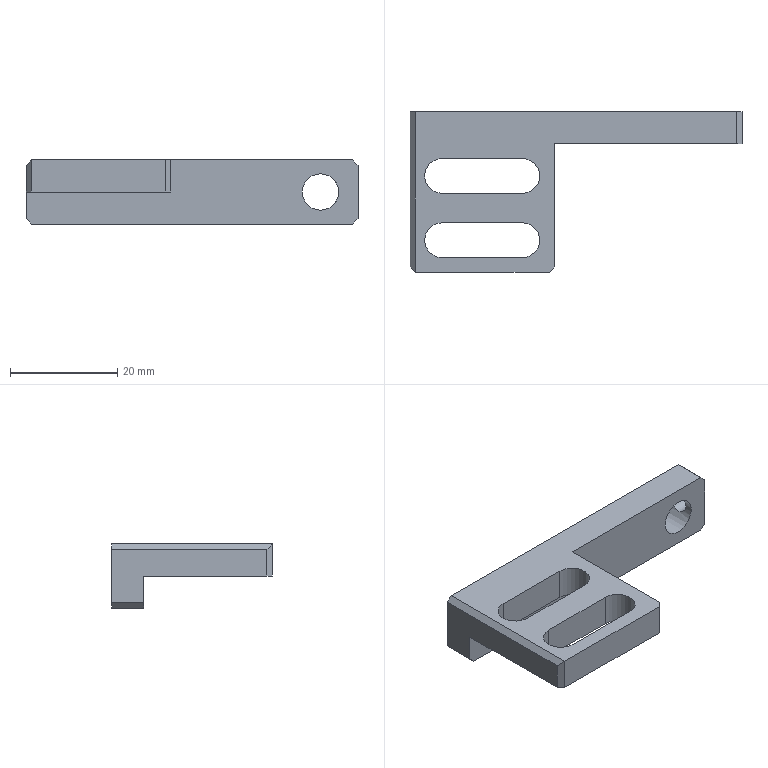NC program | NX | posted with a generic post | part box 62 x 30 x 12 mm
Lines 1128 to 2452 of 2452:
(ZLEVEL_PROFILE , TOOL : D4)
N2230 T11 M6
N2232 G54
N2234 G17 G0 G90 X11.003 Y1.75 S9500 M3
N2236 G43 Z30. H11
N2238 Z-5.
N2240 G94 G1 X25.158 Z-5.742 F1500.
N2242 X25.529 Y1.856 Z-5.762
N2244 X25.85 Y2.07 Z-5.782
N2246 X26.091 Y2.37 Z-5.802
N2248 X26.231 Y2.729 Z-5.823
N2250 X26.255 Y3.114 Z-5.843
N2252 X26.162 Y3.488 Z-5.863
N2254 X26.003 Y3.762 Z-5.88
N2256 X25.769 Y3.998 Z-5.897
N2258 X25.48 Y4.165 Z-5.915
N2260 X25.158 Y4.25 Z-5.932
N2262 X17.5 Z-6.333
N2264 X10.
N2266 G3 X8.75 Y3. R1.25
N2268 X10. Y1.75 R1.25
N2270 G1 X25.
N2272 G3 X26.25 Y3. R1.25
N2274 X25. Y4.25 R1.25
N2276 G1 X17.5
N2278 X10.198 Z-6.461
N2280 X10.058 Z-6.463
N2282 X9.918 Y4.239 Z-6.466
N2284 X9.716 Y4.209 Z-6.469
N2286 X9.643 Y4.193 Z-6.471
N2288 X9.51 Y4.143 Z-6.473
N2290 X9.388 Y4.081 Z-6.475
N2292 X9.242 Y3.984 Z-6.479
N2294 X9.16 Y3.92 Z-6.48
N2296 X9.063 Y3.818 Z-6.483
N2298 X8.979 Y3.708 Z-6.485
N2300 X8.89 Y3.557 Z-6.488
N2302 X8.844 Y3.464 Z-6.49
N2304 X8.804 Y3.335 Z-6.493
N2306 X8.773 Y3.194 Z-6.495
N2308 X8.752 Y3.075 Z-6.497
N2310 X8.753 Y2.915 Z-6.5
N2312 X8.803 Y2.64 Z-6.505
N2314 X8.913 Y2.382 Z-6.51
N2316 X8.983 Y2.287 Z-6.512
N2318 X9.084 Y2.161 Z-6.515
N2320 X9.205 Y2.045 Z-6.518
N2322 X9.292 Y1.975 Z-6.52
N2324 X9.416 Y1.903 Z-6.522
N2326 X9.54 Y1.846 Z-6.525
N2328 X9.696 Y1.795 Z-6.527
N2330 X9.808 Y1.77 Z-6.529
N2332 X9.947 Y1.758 Z-6.532
N2334 X10.087 Y1.75 Z-6.534
N2336 X17.67 Z-6.667
N2338 X25.
N2340 G3 X26.25 Y3. R1.25
N2342 X25. Y4.25 R1.25
N2344 G1 X17.5
N2346 X10.198 Z-6.794
N2348 X10.058 Z-6.797
N2350 X9.918 Y4.239 Z-6.799
N2352 X9.716 Y4.209 Z-6.803
N2354 X9.643 Y4.193 Z-6.804
N2356 X9.51 Y4.143 Z-6.806
N2358 X9.388 Y4.081 Z-6.809
N2360 X9.242 Y3.984 Z-6.812
N2362 X9.16 Y3.92 Z-6.814
N2364 X9.063 Y3.818 Z-6.816
N2366 X8.979 Y3.708 Z-6.819
N2368 X8.89 Y3.557 Z-6.822
N2370 X8.844 Y3.464 Z-6.824
N2372 X8.804 Y3.335 Z-6.826
N2374 X8.773 Y3.194 Z-6.828
N2376 X8.752 Y3.075 Z-6.831
N2378 X8.753 Y2.915 Z-6.833
N2380 X8.803 Y2.64 Z-6.838
N2382 X8.913 Y2.382 Z-6.843
N2384 X8.983 Y2.287 Z-6.845
N2386 X9.084 Y2.161 Z-6.848
N2388 X9.205 Y2.045 Z-6.851
N2390 X9.292 Y1.975 Z-6.853
N2392 X9.416 Y1.903 Z-6.855
N2394 X9.54 Y1.846 Z-6.858
N2396 X9.695 Y1.795 Z-6.861
N2398 X9.808 Y1.77 Z-6.863
N2400 X9.947 Y1.758 Z-6.865
N2402 X10.087 Y1.75 Z-6.868
N2404 X17.67 Z-7.
N2406 X25.
N2408 G3 X26.25 Y3. R1.25
N2410 X25. Y4.25 R1.25
N2412 G1 X17.5
N2414 X10.198 Z-7.127
N2416 X10.058 Z-7.13
N2418 X9.918 Y4.239 Z-7.132
N2420 X9.716 Y4.209 Z-7.136
N2422 X9.643 Y4.193 Z-7.137
N2424 X9.51 Y4.143 Z-7.14
N2426 X9.388 Y4.081 Z-7.142
N2428 X9.242 Y3.984 Z-7.145
N2430 X9.16 Y3.92 Z-7.147
N2432 X9.064 Y3.818 Z-7.15
N2434 X8.979 Y3.708 Z-7.152
N2436 X8.89 Y3.557 Z-7.155
N2438 X8.844 Y3.464 Z-7.157
N2440 X8.804 Y3.335 Z-7.159
N2442 X8.773 Y3.194 Z-7.162
N2444 X8.752 Y3.075 Z-7.164
N2446 X8.753 Y2.915 Z-7.167
N2448 X8.803 Y2.64 Z-7.172
N2450 X8.913 Y2.382 Z-7.176
N2452 X8.983 Y2.287 Z-7.179
N2454 X9.084 Y2.161 Z-7.181
N2456 X9.205 Y2.045 Z-7.184
N2458 X9.292 Y1.975 Z-7.186
N2460 X9.416 Y1.903 Z-7.189
N2462 X9.54 Y1.846 Z-7.191
N2464 X9.695 Y1.795 Z-7.194
N2466 X9.808 Y1.77 Z-7.196
N2468 X9.947 Y1.758 Z-7.199
N2470 X10.087 Y1.75 Z-7.201
N2472 X17.67 Z-7.333
N2474 X25.
N2476 G3 X26.25 Y3. R1.25
N2478 X25. Y4.25 R1.25
N2480 G1 X17.5
N2482 X10.198 Z-7.461
N2484 X10.058 Z-7.463
N2486 X9.918 Y4.239 Z-7.466
N2488 X9.716 Y4.209 Z-7.469
N2490 X9.643 Y4.193 Z-7.471
N2492 X9.51 Y4.143 Z-7.473
N2494 X9.388 Y4.081 Z-7.475
N2496 X9.242 Y3.984 Z-7.479
N2498 X9.16 Y3.92 Z-7.48
N2500 X9.064 Y3.818 Z-7.483
N2502 X8.979 Y3.708 Z-7.485
N2504 X8.89 Y3.557 Z-7.488
N2506 X8.844 Y3.464 Z-7.49
N2508 X8.804 Y3.335 Z-7.493
N2510 X8.773 Y3.194 Z-7.495
N2512 X8.752 Y3.075 Z-7.497
N2514 X8.753 Y2.915 Z-7.5
N2516 X8.803 Y2.64 Z-7.505
N2518 X8.913 Y2.382 Z-7.51
N2520 X8.983 Y2.287 Z-7.512
N2522 X9.084 Y2.161 Z-7.515
N2524 X9.205 Y2.045 Z-7.518
N2526 X9.292 Y1.975 Z-7.52
N2528 X9.416 Y1.903 Z-7.522
N2530 X9.54 Y1.846 Z-7.525
N2532 X9.695 Y1.795 Z-7.527
N2534 X9.808 Y1.77 Z-7.529
N2536 X9.947 Y1.758 Z-7.532
N2538 X10.087 Y1.75 Z-7.534
N2540 X17.67 Z-7.667
N2542 X25.
N2544 G3 X26.25 Y3. R1.25
N2546 X25. Y4.25 R1.25
N2548 G1 X17.5
N2550 X10.198 Z-7.794
N2552 X10.058 Z-7.797
N2554 X9.918 Y4.239 Z-7.799
N2556 X9.716 Y4.209 Z-7.803
N2558 X9.643 Y4.193 Z-7.804
N2560 X9.51 Y4.143 Z-7.806
N2562 X9.388 Y4.081 Z-7.809
N2564 X9.242 Y3.984 Z-7.812
N2566 X9.16 Y3.92 Z-7.814
N2568 X9.064 Y3.818 Z-7.816
N2570 X8.979 Y3.708 Z-7.819
N2572 X8.889 Y3.558 Z-7.822
N2574 X8.844 Y3.464 Z-7.824
N2576 X8.802 Y3.332 Z-7.826
N2578 X8.773 Y3.194 Z-7.828
N2580 X8.752 Y3.072 Z-7.831
N2582 X8.753 Y2.915 Z-7.833
N2584 X8.803 Y2.64 Z-7.838
N2586 X8.913 Y2.382 Z-7.843
N2588 X8.983 Y2.287 Z-7.845
N2590 X9.084 Y2.161 Z-7.848
N2592 X9.205 Y2.045 Z-7.851
N2594 X9.292 Y1.975 Z-7.853
N2596 X9.416 Y1.903 Z-7.855
N2598 X9.54 Y1.846 Z-7.858
N2600 X9.695 Y1.795 Z-7.861
N2602 X9.808 Y1.77 Z-7.863
N2604 X9.947 Y1.758 Z-7.865
N2606 X10.087 Y1.75 Z-7.868
N2608 X17.67 Z-8.
N2610 X25.
N2612 G3 X26.25 Y3. R1.25
N2614 X25. Y4.25 R1.25
N2616 G1 X17.5
N2618 X10.198 Z-8.127
N2620 X10.058 Z-8.13
N2622 X9.918 Y4.239 Z-8.132
N2624 X9.716 Y4.209 Z-8.136
N2626 X9.643 Y4.193 Z-8.137
N2628 X9.51 Y4.143 Z-8.14
N2630 X9.388 Y4.081 Z-8.142
N2632 X9.241 Y3.985 Z-8.145
N2634 X9.16 Y3.92 Z-8.147
N2636 X9.061 Y3.815 Z-8.15
N2638 X8.979 Y3.708 Z-8.152
N2640 X8.89 Y3.557 Z-8.155
N2642 X8.844 Y3.464 Z-8.157
N2644 X8.803 Y3.336 Z-8.159
N2646 X8.773 Y3.194 Z-8.162
N2648 X8.752 Y3.073 Z-8.164
N2650 X8.753 Y2.915 Z-8.167
N2652 X8.803 Y2.64 Z-8.172
N2654 X8.913 Y2.382 Z-8.176
N2656 X8.983 Y2.287 Z-8.179
N2658 X9.084 Y2.161 Z-8.181
N2660 X9.205 Y2.045 Z-8.184
N2662 X9.292 Y1.975 Z-8.186
N2664 X9.416 Y1.903 Z-8.189
N2666 X9.54 Y1.846 Z-8.191
N2668 X9.695 Y1.795 Z-8.194
N2670 X9.808 Y1.77 Z-8.196
N2672 X9.947 Y1.758 Z-8.199
N2674 X10.087 Y1.75 Z-8.201
N2676 X17.67 Z-8.333
N2678 X25.
N2680 G3 X26.25 Y3. R1.25
N2682 X25. Y4.25 R1.25
N2684 G1 X17.5
N2686 X10.198 Z-8.461
N2688 X10.058 Z-8.463
N2690 X9.918 Y4.239 Z-8.466
N2692 X9.716 Y4.209 Z-8.469
N2694 X9.643 Y4.193 Z-8.471
N2696 X9.51 Y4.143 Z-8.473
N2698 X9.388 Y4.081 Z-8.475
N2700 X9.241 Y3.985 Z-8.479
N2702 X9.16 Y3.92 Z-8.48
N2704 X9.061 Y3.815 Z-8.483
N2706 X8.979 Y3.708 Z-8.485
N2708 X8.89 Y3.557 Z-8.488
N2710 X8.844 Y3.464 Z-8.49
N2712 X8.803 Y3.336 Z-8.493
N2714 X8.773 Y3.194 Z-8.495
N2716 X8.752 Y3.073 Z-8.497
N2718 X8.753 Y2.915 Z-8.5
N2720 X8.803 Y2.64 Z-8.505
N2722 X8.913 Y2.382 Z-8.51
N2724 X8.983 Y2.287 Z-8.512
N2726 X9.084 Y2.161 Z-8.515
N2728 X9.205 Y2.045 Z-8.518
N2730 X9.292 Y1.975 Z-8.52
N2732 X9.416 Y1.903 Z-8.522
N2734 X9.54 Y1.846 Z-8.525
N2736 X9.695 Y1.795 Z-8.527
N2738 X9.808 Y1.77 Z-8.529
N2740 X9.947 Y1.758 Z-8.532
N2742 X10.087 Y1.75 Z-8.534
N2744 X17.67 Z-8.667
N2746 X25.
N2748 G3 X26.25 Y3. R1.25
N2750 X25. Y4.25 R1.25
N2752 G1 X17.5
N2754 X10.198 Z-8.794
N2756 X10.058 Z-8.797
N2758 X9.918 Y4.239 Z-8.799
N2760 X9.716 Y4.209 Z-8.803
N2762 X9.643 Y4.193 Z-8.804
N2764 X9.51 Y4.143 Z-8.806
N2766 X9.388 Y4.081 Z-8.809
N2768 X9.242 Y3.985 Z-8.812
N2770 X9.16 Y3.92 Z-8.814
N2772 X9.061 Y3.815 Z-8.816
N2774 X8.979 Y3.708 Z-8.819
N2776 X8.89 Y3.557 Z-8.822
N2778 X8.844 Y3.464 Z-8.824
N2780 X8.803 Y3.336 Z-8.826
N2782 X8.773 Y3.194 Z-8.828
N2784 X8.752 Y3.073 Z-8.831
N2786 X8.753 Y2.915 Z-8.833
N2788 X8.803 Y2.64 Z-8.838
N2790 X8.913 Y2.382 Z-8.843
N2792 X8.983 Y2.287 Z-8.845
N2794 X9.084 Y2.161 Z-8.848
N2796 X9.205 Y2.045 Z-8.851
N2798 X9.292 Y1.975 Z-8.853
N2800 X9.416 Y1.903 Z-8.855
N2802 X9.54 Y1.846 Z-8.858
N2804 X9.695 Y1.795 Z-8.861
N2806 X9.808 Y1.77 Z-8.863
N2808 X9.947 Y1.758 Z-8.865
N2810 X10.087 Y1.75 Z-8.868
N2812 X17.67 Z-9.
N2814 X25.
N2816 G3 X26.25 Y3. R1.25
N2818 X25. Y4.25 R1.25
N2820 G1 X17.5
N2822 X10.198 Z-9.127
N2824 X10.058 Z-9.13
N2826 X9.918 Y4.239 Z-9.132
N2828 X9.716 Y4.209 Z-9.136
N2830 X9.643 Y4.193 Z-9.137
N2832 X9.51 Y4.143 Z-9.14
N2834 X9.388 Y4.081 Z-9.142
N2836 X9.242 Y3.985 Z-9.145
N2838 X9.16 Y3.92 Z-9.147
N2840 X9.061 Y3.815 Z-9.15
N2842 X8.979 Y3.708 Z-9.152
N2844 X8.89 Y3.557 Z-9.155
N2846 X8.844 Y3.464 Z-9.157
N2848 X8.803 Y3.336 Z-9.159
N2850 X8.773 Y3.194 Z-9.162
N2852 X8.752 Y3.073 Z-9.164
N2854 X8.753 Y2.915 Z-9.167
N2856 X8.803 Y2.64 Z-9.172
N2858 X8.913 Y2.382 Z-9.176
N2860 X8.983 Y2.287 Z-9.179
N2862 X9.084 Y2.161 Z-9.181
N2864 X9.205 Y2.045 Z-9.184
N2866 X9.292 Y1.975 Z-9.186
N2868 X9.416 Y1.903 Z-9.189
N2870 X9.54 Y1.846 Z-9.191
N2872 X9.695 Y1.795 Z-9.194
N2874 X9.808 Y1.77 Z-9.196
N2876 X9.947 Y1.758 Z-9.199
N2878 X10.087 Y1.75 Z-9.201
N2880 X17.67 Z-9.333
N2882 X25.
N2884 G3 X26.25 Y3. R1.25
N2886 X25. Y4.25 R1.25
N2888 G1 X17.5
N2890 X10.198 Z-9.461
N2892 X10.058 Z-9.463
N2894 X9.918 Y4.239 Z-9.466
N2896 X9.716 Y4.209 Z-9.469
N2898 X9.643 Y4.193 Z-9.471
N2900 X9.51 Y4.143 Z-9.473
N2902 X9.388 Y4.081 Z-9.475
N2904 X9.242 Y3.985 Z-9.479
N2906 X9.16 Y3.92 Z-9.48
N2908 X9.061 Y3.815 Z-9.483
N2910 X8.979 Y3.708 Z-9.485
N2912 X8.89 Y3.557 Z-9.488
N2914 X8.844 Y3.464 Z-9.49
N2916 X8.803 Y3.336 Z-9.493
N2918 X8.773 Y3.194 Z-9.495
N2920 X8.752 Y3.073 Z-9.497
N2922 X8.753 Y2.915 Z-9.5
N2924 X8.803 Y2.64 Z-9.505
N2926 X8.913 Y2.382 Z-9.51
N2928 X8.983 Y2.287 Z-9.512
N2930 X9.084 Y2.161 Z-9.515
N2932 X9.205 Y2.045 Z-9.518
N2934 X9.292 Y1.975 Z-9.52
N2936 X9.416 Y1.903 Z-9.522
N2938 X9.54 Y1.846 Z-9.525
N2940 X9.695 Y1.795 Z-9.527
N2942 X9.808 Y1.77 Z-9.529
N2944 X9.947 Y1.758 Z-9.532
N2946 X10.087 Y1.75 Z-9.534
N2948 X17.67 Z-9.667
N2950 X25.
N2952 G3 X26.25 Y3. R1.25
N2954 X25. Y4.25 R1.25
N2956 G1 X17.5
N2958 X10.198 Z-9.794
N2960 X10.058 Z-9.797
N2962 X9.918 Y4.239 Z-9.799
N2964 X9.716 Y4.209 Z-9.803
N2966 X9.643 Y4.193 Z-9.804
N2968 X9.51 Y4.143 Z-9.806
N2970 X9.388 Y4.081 Z-9.809
N2972 X9.242 Y3.985 Z-9.812
N2974 X9.16 Y3.92 Z-9.814
N2976 X9.061 Y3.815 Z-9.816
N2978 X8.979 Y3.708 Z-9.819
N2980 X8.889 Y3.557 Z-9.822
N2982 X8.844 Y3.464 Z-9.824
N2984 X8.802 Y3.332 Z-9.826
N2986 X8.773 Y3.194 Z-9.828
N2988 X8.752 Y3.072 Z-9.831
N2990 X8.753 Y2.915 Z-9.833
N2992 X8.803 Y2.64 Z-9.838
N2994 X8.913 Y2.382 Z-9.843
N2996 X8.983 Y2.287 Z-9.845
N2998 X9.084 Y2.161 Z-9.848
N3000 X9.205 Y2.045 Z-9.851
N3002 X9.292 Y1.975 Z-9.853
N3004 X9.415 Y1.903 Z-9.855
N3006 X9.54 Y1.846 Z-9.858
N3008 X9.695 Y1.795 Z-9.861
N3010 X9.808 Y1.77 Z-9.863
N3012 X9.947 Y1.758 Z-9.865
N3014 X10.087 Y1.75 Z-9.868
N3016 X17.67 Z-10.
N3018 X25.
N3020 G3 X26.25 Y3. R1.25
N3022 X25. Y4.25 R1.25
N3024 G1 X17.5
N3026 X10.198 Z-10.127
N3028 X10.058 Z-10.13
N3030 X9.918 Y4.239 Z-10.132
N3032 X9.716 Y4.209 Z-10.136
N3034 X9.643 Y4.193 Z-10.137
N3036 X9.51 Y4.143 Z-10.14
N3038 X9.388 Y4.081 Z-10.142
N3040 X9.242 Y3.985 Z-10.145
N3042 X9.16 Y3.92 Z-10.147
N3044 X9.061 Y3.815 Z-10.15
N3046 X8.979 Y3.708 Z-10.152
N3048 X8.889 Y3.557 Z-10.155
N3050 X8.844 Y3.464 Z-10.157
N3052 X8.802 Y3.332 Z-10.159
N3054 X8.773 Y3.194 Z-10.162
N3056 X8.752 Y3.072 Z-10.164
N3058 X8.753 Y2.915 Z-10.167
N3060 X8.803 Y2.64 Z-10.172
N3062 X8.913 Y2.382 Z-10.176
N3064 X8.983 Y2.287 Z-10.179
N3066 X9.084 Y2.161 Z-10.181
N3068 X9.205 Y2.045 Z-10.184
N3070 X9.292 Y1.975 Z-10.186
N3072 X9.415 Y1.903 Z-10.189
N3074 X9.54 Y1.846 Z-10.191
N3076 X9.695 Y1.795 Z-10.194
N3078 X9.808 Y1.77 Z-10.196
N3080 X9.947 Y1.758 Z-10.199
N3082 X10.087 Y1.75 Z-10.201
N3084 X17.67 Z-10.333
N3086 X25.
N3088 G3 X26.25 Y3. R1.25
N3090 X25. Y4.25 R1.25
N3092 G1 X17.5
N3094 X10.198 Z-10.461
N3096 X10.058 Z-10.463
N3098 X9.918 Y4.239 Z-10.466
N3100 X9.716 Y4.209 Z-10.469
N3102 X9.643 Y4.193 Z-10.471
N3104 X9.51 Y4.143 Z-10.473
N3106 X9.388 Y4.081 Z-10.475
N3108 X9.242 Y3.985 Z-10.479
N3110 X9.16 Y3.92 Z-10.48
N3112 X9.061 Y3.815 Z-10.483
N3114 X8.979 Y3.708 Z-10.485
N3116 X8.889 Y3.557 Z-10.488
N3118 X8.844 Y3.464 Z-10.49
N3120 X8.802 Y3.332 Z-10.493
N3122 X8.773 Y3.194 Z-10.495
N3124 X8.752 Y3.072 Z-10.497
N3126 X8.753 Y2.915 Z-10.5
N3128 X8.803 Y2.64 Z-10.505
N3130 X8.913 Y2.382 Z-10.51
N3132 X8.983 Y2.287 Z-10.512
N3134 X9.084 Y2.161 Z-10.515
N3136 X9.205 Y2.045 Z-10.518
N3138 X9.292 Y1.975 Z-10.52
N3140 X9.415 Y1.903 Z-10.522
N3142 X9.54 Y1.846 Z-10.525
N3144 X9.695 Y1.795 Z-10.527
N3146 X9.808 Y1.77 Z-10.529
N3148 X9.947 Y1.758 Z-10.532
N3150 X10.087 Y1.75 Z-10.534
N3152 X17.67 Z-10.667
N3154 X25.
N3156 G3 X26.25 Y3. R1.25
N3158 X25. Y4.25 R1.25
N3160 G1 X17.5
N3162 X10.198 Z-10.794
N3164 X10.058 Z-10.797
N3166 X9.918 Y4.239 Z-10.799
N3168 X9.716 Y4.209 Z-10.803
N3170 X9.643 Y4.193 Z-10.804
N3172 X9.51 Y4.143 Z-10.806
N3174 X9.388 Y4.081 Z-10.809
N3176 X9.242 Y3.985 Z-10.812
N3178 X9.16 Y3.92 Z-10.814
N3180 X9.061 Y3.815 Z-10.816
N3182 X8.979 Y3.708 Z-10.819
N3184 X8.889 Y3.557 Z-10.822
N3186 X8.844 Y3.464 Z-10.824
N3188 X8.802 Y3.332 Z-10.826
N3190 X8.773 Y3.194 Z-10.828
N3192 X8.752 Y3.072 Z-10.831
N3194 X8.753 Y2.915 Z-10.833
N3196 X8.803 Y2.64 Z-10.838
N3198 X8.913 Y2.382 Z-10.843
N3200 X8.983 Y2.287 Z-10.845
N3202 X9.084 Y2.161 Z-10.848
N3204 X9.205 Y2.045 Z-10.851
N3206 X9.292 Y1.975 Z-10.853
N3208 X9.415 Y1.903 Z-10.855
N3210 X9.54 Y1.846 Z-10.858
N3212 X9.695 Y1.795 Z-10.861
N3214 X9.808 Y1.77 Z-10.863
N3216 X9.947 Y1.758 Z-10.865
N3218 X10.087 Y1.75 Z-10.868
N3220 X17.67 Z-11.
N3222 X25.
N3224 G3 X26.25 Y3. R1.25
N3226 X25. Y4.25 R1.25
N3228 G1 X17.5
N3230 X10.198 Z-11.127
N3232 X10.058 Z-11.13
N3234 X9.918 Y4.239 Z-11.132
N3236 X9.716 Y4.209 Z-11.136
N3238 X9.643 Y4.193 Z-11.137
N3240 X9.51 Y4.143 Z-11.14
N3242 X9.388 Y4.081 Z-11.142
N3244 X9.242 Y3.985 Z-11.145
N3246 X9.16 Y3.92 Z-11.147
N3248 X9.061 Y3.815 Z-11.15
N3250 X8.979 Y3.708 Z-11.152
N3252 X8.889 Y3.557 Z-11.155
N3254 X8.844 Y3.464 Z-11.157
N3256 X8.802 Y3.332 Z-11.159
N3258 X8.773 Y3.194 Z-11.162
N3260 X8.752 Y3.072 Z-11.164
N3262 X8.753 Y2.915 Z-11.167
N3264 X8.803 Y2.64 Z-11.172
N3266 X8.913 Y2.382 Z-11.176
N3268 X8.983 Y2.287 Z-11.179
N3270 X9.084 Y2.161 Z-11.181
N3272 X9.205 Y2.045 Z-11.184
N3274 X9.292 Y1.975 Z-11.186
N3276 X9.415 Y1.903 Z-11.189
N3278 X9.54 Y1.846 Z-11.191
N3280 X9.695 Y1.795 Z-11.194
N3282 X9.808 Y1.77 Z-11.196
N3284 X9.947 Y1.758 Z-11.199
N3286 X10.087 Y1.75 Z-11.201
N3288 X17.67 Z-11.333
N3290 X25.
N3292 G3 X26.25 Y3. R1.25
N3294 X25. Y4.25 R1.25
N3296 G1 X17.5
N3298 X10.198 Z-11.461
N3300 X10.058 Z-11.463
N3302 X9.918 Y4.239 Z-11.466
N3304 X9.716 Y4.209 Z-11.469
N3306 X9.643 Y4.193 Z-11.471
N3308 X9.51 Y4.143 Z-11.473
N3310 X9.388 Y4.081 Z-11.475
N3312 X9.242 Y3.985 Z-11.479
N3314 X9.16 Y3.92 Z-11.48
N3316 X9.061 Y3.815 Z-11.483
N3318 X8.979 Y3.708 Z-11.485
N3320 X8.889 Y3.557 Z-11.488
N3322 X8.844 Y3.464 Z-11.49
N3324 X8.802 Y3.332 Z-11.493
N3326 X8.773 Y3.194 Z-11.495
N3328 X8.752 Y3.072 Z-11.497
N3330 X8.753 Y2.915 Z-11.5
N3332 X8.803 Y2.64 Z-11.505
N3334 X8.913 Y2.382 Z-11.51
N3336 X8.983 Y2.287 Z-11.512
N3338 X9.084 Y2.161 Z-11.515
N3340 X9.205 Y2.045 Z-11.518
N3342 X9.292 Y1.975 Z-11.52
N3344 X9.415 Y1.903 Z-11.522
N3346 X9.54 Y1.846 Z-11.525
N3348 X9.695 Y1.795 Z-11.527
N3350 X9.808 Y1.77 Z-11.529
N3352 X9.947 Y1.758 Z-11.532
N3354 X10.087 Y1.75 Z-11.534
N3356 X17.67 Z-11.667
N3358 X25.
N3360 G3 X26.25 Y3. R1.25
N3362 X25. Y4.25 R1.25
N3364 G1 X17.5
N3366 X10.198 Z-11.794
N3368 X10.058 Z-11.797
N3370 X9.918 Y4.239 Z-11.799
N3372 X9.716 Y4.209 Z-11.803
N3374 X9.643 Y4.193 Z-11.804
N3376 X9.51 Y4.143 Z-11.806
N3378 X9.388 Y4.081 Z-11.809
N3380 X9.242 Y3.985 Z-11.812
N3382 X9.16 Y3.92 Z-11.814
N3384 X9.061 Y3.815 Z-11.816
N3386 X8.979 Y3.708 Z-11.819
N3388 X8.889 Y3.557 Z-11.822
N3390 X8.844 Y3.464 Z-11.824
N3392 X8.802 Y3.332 Z-11.826
N3394 X8.773 Y3.194 Z-11.828
N3396 X8.752 Y3.072 Z-11.831
N3398 X8.753 Y2.915 Z-11.833
N3400 X8.803 Y2.64 Z-11.838
N3402 X8.913 Y2.382 Z-11.843
N3404 X8.983 Y2.287 Z-11.845
N3406 X9.084 Y2.161 Z-11.848
N3408 X9.205 Y2.045 Z-11.851
N3410 X9.292 Y1.975 Z-11.853
N3412 X9.415 Y1.903 Z-11.855
N3414 X9.54 Y1.846 Z-11.858
N3416 X9.695 Y1.795 Z-11.861
N3418 X9.808 Y1.77 Z-11.863
N3420 X9.947 Y1.758 Z-11.865
N3422 X10.087 Y1.75 Z-11.868
N3424 X17.67 Z-12.
N3426 X25.
N3428 G3 X26.25 Y3. R1.25
N3430 X25. Y4.25 R1.25
N3432 G1 X10.
N3434 G3 X8.75 Y3. R1.25
N3436 X10. Y1.75 R1.25
N3438 G1 X17.67
N3440 Z-11.
N3442 G0 Z30.
N3444 X24. Y-7.75
N3446 Z-5.
N3448 G1 X9.842 Z-5.742
N3450 X9.479 Y-7.853 Z-5.762
N3452 X9.162 Y-8.059 Z-5.782
N3454 X8.921 Y-8.349 Z-5.801
N3456 X8.793 Y-8.639 Z-5.818
N3458 X8.742 Y-9.071 Z-5.841
N3460 X8.841 Y-9.495 Z-5.864
N3462 X9.079 Y-9.859 Z-5.886
N3464 X9.426 Y-10.122 Z-5.909
N3466 X9.842 Y-10.25 Z-5.932
N3468 X17.5 Z-6.333
N3470 X25.
N3472 G3 X26.25 Y-9. R1.25
N3474 X25. Y-7.75 R1.25
N3476 G1 X10.
N3478 G3 X8.75 Y-9. R1.25
N3480 X10. Y-10.25 R1.25
N3482 G1 X17.5
N3484 X24.802 Z-6.461
N3486 X24.942 Z-6.463
N3488 X25.082 Y-10.239 Z-6.466
N3490 X25.284 Y-10.209 Z-6.469
N3492 X25.357 Y-10.193 Z-6.471
N3494 X25.49 Y-10.143 Z-6.473
N3496 X25.612 Y-10.081 Z-6.475
N3498 X25.758 Y-9.984 Z-6.479
N3500 X25.84 Y-9.92 Z-6.48
N3502 X25.937 Y-9.818 Z-6.483
N3504 X26.021 Y-9.708 Z-6.485
N3506 X26.11 Y-9.557 Z-6.488
N3508 X26.156 Y-9.464 Z-6.49
N3510 X26.199 Y-9.33 Z-6.493
N3512 X26.227 Y-9.194 Z-6.495
N3514 X26.242 Y-9.02 Z-6.498
N3516 Y-8.916 Z-6.5
N3518 X26.223 Y-8.776 Z-6.502
N3520 X26.189 Y-8.642 Z-6.505
N3522 X26.127 Y-8.478 Z-6.508
N3524 X26.082 Y-8.384 Z-6.51
N3526 X26.004 Y-8.267 Z-6.512
N3528 X25.916 Y-8.161 Z-6.515
N3530 X25.789 Y-8.041 Z-6.518
N3532 X25.708 Y-7.975 Z-6.52
N3534 X25.586 Y-7.904 Z-6.522
N3536 X25.46 Y-7.846 Z-6.525
N3538 X25.305 Y-7.795 Z-6.527
N3540 X25.192 Y-7.77 Z-6.529
N3542 X25.053 Y-7.758 Z-6.532
N3544 X24.913 Y-7.75 Z-6.534
N3546 X17.33 Z-6.667
N3548 X10.
N3550 G3 X8.75 Y-9. R1.25
N3552 X10. Y-10.25 R1.25
N3554 G1 X17.5
N3556 X24.802 Z-6.794
N3558 X24.942 Z-6.797
N3560 X25.082 Y-10.239 Z-6.799
N3562 X25.284 Y-10.209 Z-6.803
N3564 X25.357 Y-10.193 Z-6.804
N3566 X25.49 Y-10.143 Z-6.806
N3568 X25.612 Y-10.081 Z-6.809
N3570 X25.758 Y-9.984 Z-6.812
N3572 X25.84 Y-9.92 Z-6.814
N3574 X25.937 Y-9.818 Z-6.816
N3576 X26.021 Y-9.708 Z-6.819
N3578 X26.11 Y-9.557 Z-6.822
N3580 X26.156 Y-9.464 Z-6.824
N3582 X26.199 Y-9.33 Z-6.826
N3584 X26.227 Y-9.194 Z-6.828
N3586 X26.242 Y-9.02 Z-6.831
N3588 Y-8.916 Z-6.833
N3590 X26.223 Y-8.776 Z-6.836
N3592 X26.189 Y-8.642 Z-6.838
N3594 X26.127 Y-8.478 Z-6.841
N3596 X26.082 Y-8.384 Z-6.843
N3598 X26.004 Y-8.267 Z-6.846
N3600 X25.916 Y-8.161 Z-6.848
N3602 X25.789 Y-8.041 Z-6.851
N3604 X25.708 Y-7.975 Z-6.853
N3606 X25.586 Y-7.904 Z-6.855
N3608 X25.46 Y-7.846 Z-6.858
N3610 X25.305 Y-7.795 Z-6.861
N3612 X25.192 Y-7.77 Z-6.863
N3614 X25.053 Y-7.758 Z-6.865
N3616 X24.913 Y-7.75 Z-6.868
N3618 X17.33 Z-7.
N3620 X10.
N3622 G3 X8.75 Y-9. R1.25
N3624 X10. Y-10.25 R1.25
N3626 G1 X17.5
N3628 X24.802 Z-7.127
N3630 X24.942 Z-7.13
N3632 X25.082 Y-10.239 Z-7.132
N3634 X25.284 Y-10.209 Z-7.136
N3636 X25.357 Y-10.193 Z-7.137
N3638 X25.49 Y-10.143 Z-7.14
N3640 X25.612 Y-10.081 Z-7.142
N3642 X25.758 Y-9.984 Z-7.145
N3644 X25.84 Y-9.92 Z-7.147
N3646 X25.936 Y-9.818 Z-7.15
N3648 X26.021 Y-9.708 Z-7.152
N3650 X26.11 Y-9.557 Z-7.155
N3652 X26.156 Y-9.464 Z-7.157
N3654 X26.199 Y-9.33 Z-7.159
N3656 X26.227 Y-9.194 Z-7.162
N3658 X26.242 Y-9.02 Z-7.165
N3660 Y-8.916 Z-7.167
N3662 X26.223 Y-8.776 Z-7.169
N3664 X26.189 Y-8.642 Z-7.172
N3666 X26.127 Y-8.478 Z-7.175
N3668 X26.082 Y-8.384 Z-7.176
N3670 X26.004 Y-8.267 Z-7.179
N3672 X25.916 Y-8.161 Z-7.181
N3674 X25.789 Y-8.041 Z-7.184
N3676 X25.708 Y-7.975 Z-7.186
N3678 X25.586 Y-7.904 Z-7.189
N3680 X25.46 Y-7.846 Z-7.191
N3682 X25.305 Y-7.795 Z-7.194
N3684 X25.192 Y-7.77 Z-7.196
N3686 X25.053 Y-7.758 Z-7.199
N3688 X24.913 Y-7.75 Z-7.201
N3690 X17.33 Z-7.333
N3692 X10.
N3694 G3 X8.75 Y-9. R1.25
N3696 X10. Y-10.25 R1.25
N3698 G1 X17.5
N3700 X24.802 Z-7.461
N3702 X24.942 Z-7.463
N3704 X25.082 Y-10.239 Z-7.466
N3706 X25.284 Y-10.209 Z-7.469
N3708 X25.357 Y-10.193 Z-7.471
N3710 X25.49 Y-10.143 Z-7.473
N3712 X25.612 Y-10.081 Z-7.475
N3714 X25.758 Y-9.984 Z-7.479
N3716 X25.84 Y-9.92 Z-7.48
N3718 X25.936 Y-9.818 Z-7.483
N3720 X26.021 Y-9.708 Z-7.485
N3722 X26.11 Y-9.557 Z-7.488
N3724 X26.156 Y-9.464 Z-7.49
N3726 X26.199 Y-9.33 Z-7.493
N3728 X26.227 Y-9.194 Z-7.495
N3730 X26.242 Y-9.02 Z-7.498
N3732 Y-8.916 Z-7.5
N3734 X26.223 Y-8.776 Z-7.502
N3736 X26.189 Y-8.642 Z-7.505
N3738 X26.127 Y-8.479 Z-7.508
N3740 X26.082 Y-8.384 Z-7.51
N3742 X26.004 Y-8.267 Z-7.512
N3744 X25.916 Y-8.161 Z-7.515
N3746 X25.789 Y-8.041 Z-7.518
N3748 X25.708 Y-7.975 Z-7.52
N3750 X25.586 Y-7.904 Z-7.522
N3752 X25.46 Y-7.846 Z-7.525
N3754 X25.305 Y-7.795 Z-7.527
N3756 X25.192 Y-7.77 Z-7.529
N3758 X25.053 Y-7.758 Z-7.532
N3760 X24.913 Y-7.75 Z-7.534
N3762 X17.33 Z-7.667
N3764 X10.
N3766 G3 X8.75 Y-9. R1.25
N3768 X10. Y-10.25 R1.25
N3770 G1 X17.5
N3772 X24.802 Z-7.794
N3774 X24.942 Z-7.797
N3776 X25.082 Y-10.239 Z-7.799
N3778 X25.284 Y-10.209 Z-7.803
N3780 X25.357 Y-10.193 Z-7.804
N3782 X25.49 Y-10.143 Z-7.806
N3784 X25.612 Y-10.081 Z-7.809
N3786 X25.758 Y-9.984 Z-7.812
N3788 X25.84 Y-9.92 Z-7.814
N3790 X25.936 Y-9.818 Z-7.816
N3792 X26.021 Y-9.708 Z-7.819
N3794 X26.111 Y-9.558 Z-7.822
N3796 X26.156 Y-9.464 Z-7.824
N3798 X26.2 Y-9.326 Z-7.826
N3800 X26.227 Y-9.194 Z-7.828
N3802 X26.242 Y-9.019 Z-7.832
N3804 Y-8.916 Z-7.833
N3806 X26.223 Y-8.776 Z-7.836
N3808 X26.189 Y-8.642 Z-7.838
N3810 X26.127 Y-8.479 Z-7.841
N3812 X26.082 Y-8.384 Z-7.843
N3814 X26.004 Y-8.267 Z-7.846
N3816 X25.916 Y-8.161 Z-7.848
N3818 X25.789 Y-8.041 Z-7.851
N3820 X25.708 Y-7.975 Z-7.853
N3822 X25.586 Y-7.904 Z-7.855
N3824 X25.46 Y-7.846 Z-7.858
N3826 X25.305 Y-7.795 Z-7.861
N3828 X25.192 Y-7.77 Z-7.863
N3830 X25.053 Y-7.758 Z-7.865
N3832 X24.913 Y-7.75 Z-7.868
N3834 X17.33 Z-8.
N3836 X10.
N3838 G3 X8.75 Y-9. R1.25
N3840 X10. Y-10.25 R1.25
N3842 G1 X17.5
N3844 X24.802 Z-8.127
N3846 X24.942 Z-8.13
N3848 X25.082 Y-10.239 Z-8.132
N3850 X25.284 Y-10.209 Z-8.136
N3852 X25.357 Y-10.193 Z-8.137
N3854 X25.49 Y-10.143 Z-8.14
N3856 X25.612 Y-10.081 Z-8.142
N3858 X25.759 Y-9.985 Z-8.145
N3860 X25.84 Y-9.92 Z-8.147
N3862 X25.939 Y-9.815 Z-8.15
N3864 X26.021 Y-9.708 Z-8.152
N3866 X26.11 Y-9.557 Z-8.155
N3868 X26.156 Y-9.464 Z-8.157
N3870 X26.199 Y-9.33 Z-8.159
N3872 X26.227 Y-9.194 Z-8.162
N3874 X26.242 Y-9.02 Z-8.165
N3876 Y-8.916 Z-8.167
N3878 X26.223 Y-8.776 Z-8.169
N3880 X26.189 Y-8.642 Z-8.172
N3882 X26.127 Y-8.479 Z-8.175
N3884 X26.082 Y-8.384 Z-8.176
N3886 X26.004 Y-8.267 Z-8.179
N3888 X25.916 Y-8.161 Z-8.181
N3890 X25.789 Y-8.041 Z-8.184
N3892 X25.708 Y-7.975 Z-8.186
N3894 X25.587 Y-7.904 Z-8.189
N3896 X25.46 Y-7.846 Z-8.191
N3898 X25.305 Y-7.795 Z-8.194
N3900 X25.192 Y-7.77 Z-8.196
N3902 X25.053 Y-7.758 Z-8.199
N3904 X24.913 Y-7.75 Z-8.201
N3906 X17.33 Z-8.333
N3908 X10.
N3910 G3 X8.75 Y-9. R1.25
N3912 X10. Y-10.25 R1.25
N3914 G1 X17.5
N3916 X24.802 Z-8.461
N3918 X24.942 Z-8.463
N3920 X25.082 Y-10.239 Z-8.466
N3922 X25.284 Y-10.209 Z-8.469
N3924 X25.357 Y-10.193 Z-8.471
N3926 X25.49 Y-10.143 Z-8.473
N3928 X25.612 Y-10.081 Z-8.475
N3930 X25.759 Y-9.985 Z-8.479
N3932 X25.84 Y-9.92 Z-8.48
N3934 X25.939 Y-9.815 Z-8.483
N3936 X26.021 Y-9.708 Z-8.485
N3938 X26.11 Y-9.557 Z-8.488
N3940 X26.156 Y-9.464 Z-8.49
N3942 X26.199 Y-9.33 Z-8.493
N3944 X26.227 Y-9.194 Z-8.495
N3946 X26.243 Y-9.02 Z-8.498
N3948 X26.242 Y-8.916 Z-8.5
N3950 X26.222 Y-8.773 Z-8.503
N3952 X26.189 Y-8.642 Z-8.505
N3954 X26.127 Y-8.478 Z-8.508
N3956 X26.082 Y-8.384 Z-8.51
N3958 X26.004 Y-8.267 Z-8.512
N3960 X25.916 Y-8.161 Z-8.515
N3962 X25.789 Y-8.041 Z-8.518
N3964 X25.708 Y-7.975 Z-8.52
N3966 X25.587 Y-7.904 Z-8.522
N3968 X25.46 Y-7.846 Z-8.525
N3970 X25.305 Y-7.795 Z-8.527
N3972 X25.192 Y-7.77 Z-8.529
N3974 X25.053 Y-7.758 Z-8.532
N3976 X24.913 Y-7.75 Z-8.534
N3978 X17.33 Z-8.667
N3980 X10.
N3982 G3 X8.75 Y-9. R1.25
N3984 X10. Y-10.25 R1.25
N3986 G1 X17.5
N3988 X24.802 Z-8.794
N3990 X24.942 Z-8.797
N3992 X25.082 Y-10.239 Z-8.799
N3994 X25.284 Y-10.209 Z-8.803
N3996 X25.357 Y-10.193 Z-8.804
N3998 X25.49 Y-10.143 Z-8.806
N4000 X25.612 Y-10.081 Z-8.809
N4002 X25.758 Y-9.985 Z-8.812
N4004 X25.84 Y-9.92 Z-8.814
N4006 X25.939 Y-9.815 Z-8.816
N4008 X26.021 Y-9.708 Z-8.819
N4010 X26.11 Y-9.557 Z-8.822
N4012 X26.156 Y-9.464 Z-8.824
N4014 X26.199 Y-9.33 Z-8.826
N4016 X26.227 Y-9.194 Z-8.828
N4018 X26.243 Y-9.02 Z-8.831
N4020 X26.242 Y-8.916 Z-8.833
N4022 X26.222 Y-8.773 Z-8.836
N4024 X26.189 Y-8.642 Z-8.838
N4026 X26.127 Y-8.478 Z-8.841
N4028 X26.082 Y-8.384 Z-8.843
N4030 X26.004 Y-8.267 Z-8.846
N4032 X25.916 Y-8.161 Z-8.848
N4034 X25.789 Y-8.041 Z-8.851
N4036 X25.708 Y-7.975 Z-8.853
N4038 X25.587 Y-7.904 Z-8.855
N4040 X25.46 Y-7.846 Z-8.858
N4042 X25.305 Y-7.795 Z-8.861
N4044 X25.192 Y-7.77 Z-8.863
N4046 X25.053 Y-7.758 Z-8.865
N4048 X24.913 Y-7.75 Z-8.868
N4050 X17.33 Z-9.
N4052 X10.
N4054 G3 X8.75 Y-9. R1.25
N4056 X10. Y-10.25 R1.25
N4058 G1 X17.5
N4060 X24.802 Z-9.127
N4062 X24.942 Z-9.13
N4064 X25.082 Y-10.239 Z-9.132
N4066 X25.284 Y-10.209 Z-9.136
N4068 X25.357 Y-10.193 Z-9.137
N4070 X25.49 Y-10.143 Z-9.14
N4072 X25.612 Y-10.081 Z-9.142
N4074 X25.758 Y-9.985 Z-9.145
N4076 X25.84 Y-9.92 Z-9.147
N4078 X25.939 Y-9.815 Z-9.15
N4080 X26.021 Y-9.708 Z-9.152
N4082 X26.11 Y-9.557 Z-9.155
N4084 X26.156 Y-9.464 Z-9.157
N4086 X26.199 Y-9.33 Z-9.159
N4088 X26.227 Y-9.194 Z-9.162
N4090 X26.243 Y-9.02 Z-9.165
N4092 X26.242 Y-8.916 Z-9.167
N4094 X26.222 Y-8.773 Z-9.169
N4096 X26.189 Y-8.642 Z-9.172
N4098 X26.127 Y-8.478 Z-9.175
N4100 X26.082 Y-8.384 Z-9.176
N4102 X26.004 Y-8.267 Z-9.179
N4104 X25.916 Y-8.161 Z-9.181
N4106 X25.789 Y-8.041 Z-9.184
N4108 X25.708 Y-7.975 Z-9.186
N4110 X25.587 Y-7.904 Z-9.189
N4112 X25.46 Y-7.846 Z-9.191
N4114 X25.305 Y-7.795 Z-9.194
N4116 X25.192 Y-7.77 Z-9.196
N4118 X25.053 Y-7.758 Z-9.199
N4120 X24.913 Y-7.75 Z-9.201
N4122 X17.33 Z-9.333
N4124 X10.
N4126 G3 X8.75 Y-9. R1.25
N4128 X10. Y-10.25 R1.25
N4130 G1 X17.5
N4132 X24.802 Z-9.461
N4134 X24.942 Z-9.463
N4136 X25.082 Y-10.239 Z-9.466
N4138 X25.284 Y-10.209 Z-9.469
N4140 X25.357 Y-10.193 Z-9.471
N4142 X25.49 Y-10.143 Z-9.473
N4144 X25.612 Y-10.081 Z-9.475
N4146 X25.758 Y-9.985 Z-9.479
N4148 X25.84 Y-9.92 Z-9.48
N4150 X25.939 Y-9.815 Z-9.483
N4152 X26.021 Y-9.708 Z-9.485
N4154 X26.11 Y-9.557 Z-9.488
N4156 X26.156 Y-9.464 Z-9.49
N4158 X26.199 Y-9.33 Z-9.493
N4160 X26.227 Y-9.194 Z-9.495
N4162 X26.243 Y-9.02 Z-9.498
N4164 X26.242 Y-8.916 Z-9.5
N4166 X26.222 Y-8.773 Z-9.503
N4168 X26.189 Y-8.642 Z-9.505
N4170 X26.127 Y-8.478 Z-9.508
N4172 X26.082 Y-8.384 Z-9.51
N4174 X26.004 Y-8.267 Z-9.512
N4176 X25.916 Y-8.161 Z-9.515
N4178 X25.789 Y-8.041 Z-9.518
N4180 X25.708 Y-7.975 Z-9.52
N4182 X25.587 Y-7.904 Z-9.522
N4184 X25.46 Y-7.846 Z-9.525
N4186 X25.305 Y-7.795 Z-9.527
N4188 X25.192 Y-7.77 Z-9.529
N4190 X25.053 Y-7.758 Z-9.532
N4192 X24.913 Y-7.75 Z-9.534
N4194 X17.33 Z-9.667
N4196 X10.
N4198 G3 X8.75 Y-9. R1.25
N4200 X10. Y-10.25 R1.25
N4202 G1 X17.5
N4204 X24.802 Z-9.794
N4206 X24.942 Z-9.797
N4208 X25.082 Y-10.239 Z-9.799
N4210 X25.284 Y-10.209 Z-9.803
N4212 X25.357 Y-10.193 Z-9.804
N4214 X25.49 Y-10.143 Z-9.806
N4216 X25.612 Y-10.081 Z-9.809
N4218 X25.758 Y-9.985 Z-9.812
N4220 X25.84 Y-9.92 Z-9.814
N4222 X25.939 Y-9.815 Z-9.816
N4224 X26.021 Y-9.708 Z-9.819
N4226 X26.111 Y-9.557 Z-9.822
N4228 X26.156 Y-9.464 Z-9.824
N4230 X26.2 Y-9.326 Z-9.826
N4232 X26.227 Y-9.194 Z-9.828
N4234 X26.242 Y-9.019 Z-9.832
N4236 Y-8.916 Z-9.833
N4238 X26.223 Y-8.776 Z-9.836
N4240 X26.189 Y-8.642 Z-9.838
N4242 X26.128 Y-8.478 Z-9.841
N4244 X26.082 Y-8.384 Z-9.843
N4246 X26.002 Y-8.265 Z-9.846
N4248 X25.916 Y-8.161 Z-9.848
N4250 X25.788 Y-8.04 Z-9.851
N4252 X25.708 Y-7.975 Z-9.853
N4254 X25.586 Y-7.904 Z-9.855
N4256 X25.46 Y-7.846 Z-9.858
N4258 X25.305 Y-7.795 Z-9.861
N4260 X25.192 Y-7.77 Z-9.863
N4262 X25.053 Y-7.758 Z-9.865
N4264 X24.913 Y-7.75 Z-9.868
N4266 X17.33 Z-10.
N4268 X10.
N4270 G3 X8.75 Y-9. R1.25
N4272 X10. Y-10.25 R1.25
N4274 G1 X17.5
N4276 X24.802 Z-10.127
N4278 X24.942 Z-10.13
N4280 X25.082 Y-10.239 Z-10.132
N4282 X25.284 Y-10.209 Z-10.136
N4284 X25.357 Y-10.193 Z-10.137
N4286 X25.49 Y-10.143 Z-10.14
N4288 X25.612 Y-10.081 Z-10.142
N4290 X25.758 Y-9.985 Z-10.145
N4292 X25.84 Y-9.92 Z-10.147
N4294 X25.939 Y-9.815 Z-10.15
N4296 X26.021 Y-9.708 Z-10.152
N4298 X26.111 Y-9.557 Z-10.155
N4300 X26.156 Y-9.464 Z-10.157
N4302 X26.2 Y-9.326 Z-10.159
N4304 X26.227 Y-9.194 Z-10.162
N4306 X26.242 Y-9.019 Z-10.165
N4308 Y-8.916 Z-10.167
N4310 X26.223 Y-8.776 Z-10.169
N4312 X26.189 Y-8.642 Z-10.172
N4314 X26.128 Y-8.478 Z-10.175
N4316 X26.082 Y-8.384 Z-10.176
N4318 X26.002 Y-8.265 Z-10.179
N4320 X25.916 Y-8.161 Z-10.181
N4322 X25.788 Y-8.04 Z-10.184
N4324 X25.708 Y-7.975 Z-10.186
N4326 X25.586 Y-7.904 Z-10.189
N4328 X25.46 Y-7.846 Z-10.191
N4330 X25.305 Y-7.795 Z-10.194
N4332 X25.192 Y-7.77 Z-10.196
N4334 X25.053 Y-7.758 Z-10.199
N4336 X24.913 Y-7.75 Z-10.201
N4338 X17.33 Z-10.333
N4340 X10.
N4342 G3 X8.75 Y-9. R1.25
N4344 X10. Y-10.25 R1.25
N4346 G1 X17.5
N4348 X24.802 Z-10.461
N4350 X24.942 Z-10.463
N4352 X25.082 Y-10.239 Z-10.466
N4354 X25.284 Y-10.209 Z-10.469
N4356 X25.357 Y-10.193 Z-10.471
N4358 X25.49 Y-10.143 Z-10.473
N4360 X25.612 Y-10.081 Z-10.475
N4362 X25.758 Y-9.985 Z-10.479
N4364 X25.84 Y-9.92 Z-10.48
N4366 X25.939 Y-9.815 Z-10.483
N4368 X26.021 Y-9.708 Z-10.485
N4370 X26.111 Y-9.557 Z-10.488
N4372 X26.156 Y-9.464 Z-10.49
N4374 X26.2 Y-9.326 Z-10.493
N4376 X26.227 Y-9.194 Z-10.495
N4378 X26.243 Y-9.019 Z-10.498
N4380 X26.242 Y-8.916 Z-10.5
N4382 X26.222 Y-8.773 Z-10.503
N4384 X26.189 Y-8.642 Z-10.505
N4386 X26.127 Y-8.478 Z-10.508
N4388 X26.082 Y-8.384 Z-10.51
N4390 X26.004 Y-8.267 Z-10.512
N4392 X25.916 Y-8.161 Z-10.515
N4394 X25.789 Y-8.04 Z-10.518
N4396 X25.708 Y-7.975 Z-10.52
N4398 X25.583 Y-7.902 Z-10.522
N4400 X25.46 Y-7.846 Z-10.525
N4402 X25.304 Y-7.795 Z-10.527
N4404 X25.192 Y-7.77 Z-10.529
N4406 X25.053 Y-7.758 Z-10.532
N4408 X24.913 Y-7.75 Z-10.534
N4410 X17.33 Z-10.667
N4412 X10.
N4414 G3 X8.75 Y-9. R1.25
N4416 X10. Y-10.25 R1.25
N4418 G1 X17.5
N4420 X24.802 Z-10.794
N4422 X24.942 Z-10.797
N4424 X25.082 Y-10.239 Z-10.799
N4426 X25.284 Y-10.209 Z-10.803
N4428 X25.357 Y-10.193 Z-10.804
N4430 X25.49 Y-10.143 Z-10.806
N4432 X25.612 Y-10.081 Z-10.809
N4434 X25.758 Y-9.985 Z-10.812
N4436 X25.84 Y-9.92 Z-10.814
N4438 X25.939 Y-9.815 Z-10.816
N4440 X26.021 Y-9.708 Z-10.819
N4442 X26.111 Y-9.557 Z-10.822
N4444 X26.156 Y-9.464 Z-10.824
N4446 X26.2 Y-9.326 Z-10.826
N4448 X26.227 Y-9.194 Z-10.828
N4450 X26.243 Y-9.019 Z-10.832
N4452 X26.242 Y-8.916 Z-10.833
N4454 X26.222 Y-8.773 Z-10.836
N4456 X26.189 Y-8.642 Z-10.838
N4458 X26.127 Y-8.478 Z-10.841
N4460 X26.082 Y-8.384 Z-10.843
N4462 X26.004 Y-8.267 Z-10.846
N4464 X25.916 Y-8.161 Z-10.848
N4466 X25.789 Y-8.04 Z-10.851
N4468 X25.708 Y-7.975 Z-10.853
N4470 X25.583 Y-7.902 Z-10.855
N4472 X25.46 Y-7.846 Z-10.858
N4474 X25.305 Y-7.795 Z-10.861
N4476 X25.192 Y-7.77 Z-10.863
N4478 X25.053 Y-7.758 Z-10.865
N4480 X24.913 Y-7.75 Z-10.868
N4482 X17.33 Z-11.
N4484 X10.
N4486 G3 X8.75 Y-9. R1.25
N4488 X10. Y-10.25 R1.25
N4490 G1 X17.5
N4492 X24.802 Z-11.127
N4494 X24.942 Z-11.13
N4496 X25.082 Y-10.239 Z-11.132
N4498 X25.284 Y-10.209 Z-11.136
N4500 X25.357 Y-10.193 Z-11.137
N4502 X25.49 Y-10.143 Z-11.14
N4504 X25.612 Y-10.081 Z-11.142
N4506 X25.758 Y-9.985 Z-11.145
N4508 X25.84 Y-9.92 Z-11.147
N4510 X25.939 Y-9.815 Z-11.15
N4512 X26.021 Y-9.708 Z-11.152
N4514 X26.111 Y-9.557 Z-11.155
N4516 X26.156 Y-9.464 Z-11.157
N4518 X26.2 Y-9.326 Z-11.159
N4520 X26.227 Y-9.194 Z-11.162
N4522 X26.243 Y-9.019 Z-11.165
N4524 X26.242 Y-8.916 Z-11.167
N4526 X26.222 Y-8.773 Z-11.169
N4528 X26.189 Y-8.642 Z-11.172
N4530 X26.128 Y-8.478 Z-11.175
N4532 X26.082 Y-8.384 Z-11.176
N4534 X26.002 Y-8.264 Z-11.179
N4536 X25.916 Y-8.161 Z-11.181
N4538 X25.788 Y-8.04 Z-11.184
N4540 X25.708 Y-7.975 Z-11.186
N4542 X25.587 Y-7.904 Z-11.189
N4544 X25.46 Y-7.846 Z-11.191
N4546 X25.305 Y-7.796 Z-11.194
N4548 X25.192 Y-7.77 Z-11.196
N4550 X25.053 Y-7.758 Z-11.199
N4552 X24.913 Y-7.75 Z-11.201
N4554 X17.33 Z-11.333
N4556 X10.
N4558 G3 X8.75 Y-9. R1.25
N4560 X10. Y-10.25 R1.25
N4562 G1 X17.5
N4564 X24.802 Z-11.461
N4566 X24.942 Z-11.463
N4568 X25.082 Y-10.239 Z-11.466
N4570 X25.284 Y-10.209 Z-11.469
N4572 X25.357 Y-10.193 Z-11.471
N4574 X25.49 Y-10.143 Z-11.473
N4576 X25.612 Y-10.081 Z-11.475
N4578 X25.758 Y-9.985 Z-11.479
N4580 X25.84 Y-9.92 Z-11.48
N4582 X25.939 Y-9.815 Z-11.483
N4584 X26.021 Y-9.708 Z-11.485
N4586 X26.111 Y-9.557 Z-11.488
N4588 X26.156 Y-9.464 Z-11.49
N4590 X26.199 Y-9.326 Z-11.493
N4592 X26.227 Y-9.194 Z-11.495
N4594 X26.243 Y-9.019 Z-11.498
N4596 X26.242 Y-8.916 Z-11.5
N4598 X26.222 Y-8.773 Z-11.503
N4600 X26.189 Y-8.642 Z-11.505
N4602 X26.128 Y-8.478 Z-11.508
N4604 X26.082 Y-8.384 Z-11.51
N4606 X26.002 Y-8.265 Z-11.512
N4608 X25.916 Y-8.161 Z-11.515
N4610 X25.788 Y-8.04 Z-11.518
N4612 X25.708 Y-7.975 Z-11.52
N4614 X25.587 Y-7.904 Z-11.522
N4616 X25.46 Y-7.846 Z-11.525
N4618 X25.305 Y-7.796 Z-11.527
N4620 X25.192 Y-7.77 Z-11.529
N4622 X25.053 Y-7.758 Z-11.532
N4624 X24.913 Y-7.75 Z-11.534
N4626 X17.33 Z-11.667
N4628 X10.
N4630 G3 X8.75 Y-9. R1.25
N4632 X10. Y-10.25 R1.25
N4634 G1 X17.5
N4636 X24.802 Z-11.794
N4638 X24.942 Z-11.797
N4640 X25.082 Y-10.239 Z-11.799
N4642 X25.284 Y-10.209 Z-11.803
N4644 X25.357 Y-10.193 Z-11.804
N4646 X25.49 Y-10.143 Z-11.806
N4648 X25.612 Y-10.081 Z-11.809
N4650 X25.758 Y-9.985 Z-11.812
N4652 X25.84 Y-9.92 Z-11.814
N4654 X25.939 Y-9.815 Z-11.816
N4656 X26.021 Y-9.708 Z-11.819
N4658 X26.111 Y-9.557 Z-11.822
N4660 X26.156 Y-9.464 Z-11.824
N4662 X26.199 Y-9.326 Z-11.826
N4664 X26.227 Y-9.194 Z-11.828
N4666 X26.243 Y-9.019 Z-11.832
N4668 X26.242 Y-8.916 Z-11.833
N4670 X26.222 Y-8.773 Z-11.836
N4672 X26.189 Y-8.642 Z-11.838
N4674 X26.128 Y-8.478 Z-11.841
N4676 X26.082 Y-8.384 Z-11.843
N4678 X26.002 Y-8.265 Z-11.846
N4680 X25.916 Y-8.161 Z-11.848
N4682 X25.789 Y-8.04 Z-11.851
N4684 X25.708 Y-7.975 Z-11.853
N4686 X25.583 Y-7.902 Z-11.855
N4688 X25.46 Y-7.846 Z-11.858
N4690 X25.305 Y-7.795 Z-11.861
N4692 X25.192 Y-7.77 Z-11.863
N4694 X25.053 Y-7.758 Z-11.865
N4696 X24.913 Y-7.75 Z-11.868
N4698 X17.33 Z-12.
N4700 X10.
N4702 G3 X8.75 Y-9. R1.25
N4704 X10. Y-10.25 R1.25
N4706 G1 X25.
N4708 G3 X26.25 Y-9. R1.25
N4710 X25. Y-7.75 R1.25
N4712 G1 X17.33
N4714 Z-11.
N4716 G0 Z30.
N4718 M5
(PLANAR_MILL_COPY_COPY_COPY , TOOL : D6A45)
N4720 T01 M6
N4722 G54
N4724 G17 G0 G90 X0.866 Y7.6 S9500 M3
N4726 G43 Z30. H1
N4728 Z0.5
N4730 G94 G1 Z-1. F1250.
N4732 G3 X0. Y8.1 R1.
N4734 G1 X-31.
N4736 G2 X-31.9 Y9. R0.9
N4738 G1 Y15.
N4740 G2 X-31. Y15.9 R0.9
N4742 G1 X31.
N4744 G2 X31.9 Y15. R0.9
N4746 G1 Y9.
N4748 G2 X31. Y8.1 R0.9
N4750 G1 X0.
N4752 G3 X-0.866 Y7.6 R1.
N4754 G1 Z0.5
N4756 G0 Z30.
(PLANAR_MILL_COPY_COPY_COPY_COPY , TOOL : D6A45)
N4758 X33.313 Y4.908
N4760 Z-5.5
N4762 G1 Z-7.
N4764 X32.865 Y5.357
N4766 G3 X31.9 Y5.618 R1.
N4768 G1 Y-13.959
N4770 G2 X31.607 Y-14.666 R1.
N4772 G1 X30.666 Y-15.607
N4774 G2 X29.959 Y-15.9 R1.
N4776 G1 X5.041
N4778 G2 X4.334 Y-15.607 R1.
N4780 G1 X3.393 Y-14.666
N4782 G2 X3.1 Y-13.959 R1.
N4784 G1 Y5.5
N4786 G3 X2.234 Y5. R1.
N4788 G1 X1.83 Y4.3
N4790 Z-5.5
N4792 G0 Z30.
N4794 X18.77 Y4.15
N4796 Z-5.5
N4798 G1 Z-7.
N4800 X18.366 Y4.85
N4802 G3 X17.5 Y5.35 R1.
N4804 G1 X10.
N4806 G3 X7.65 Y3. R2.35
N4808 X10. Y0.65 R2.35
N4810 G1 X25.
N4812 G3 X27.35 Y3. R2.35
N4814 X25. Y5.35 R2.35
N4816 G1 X17.5
N4818 G3 X16.634 Y4.85 R1.
N4820 G1 X16.23 Y4.15
N4822 Z-5.5
N4824 G0 Z30.
N4826 Y-10.15
N4828 Z-5.5
N4830 G1 Z-7.
N4832 X16.634 Y-10.85
N4834 G3 X17.5 Y-11.35 R1.
N4836 G1 X25.
N4838 G3 X27.35 Y-9. R2.35
N4840 X25. Y-6.65 R2.35
N4842 G1 X10.
N4844 G3 X7.65 Y-9. R2.35
N4846 X10. Y-11.35 R2.35
N4848 G1 X17.5
N4850 G3 X18.366 Y-10.85 R1.
N4852 G1 X18.77 Y-10.15
N4854 Z-5.5
N4856 G0 Z30.
N4858 M5
N4860 M2